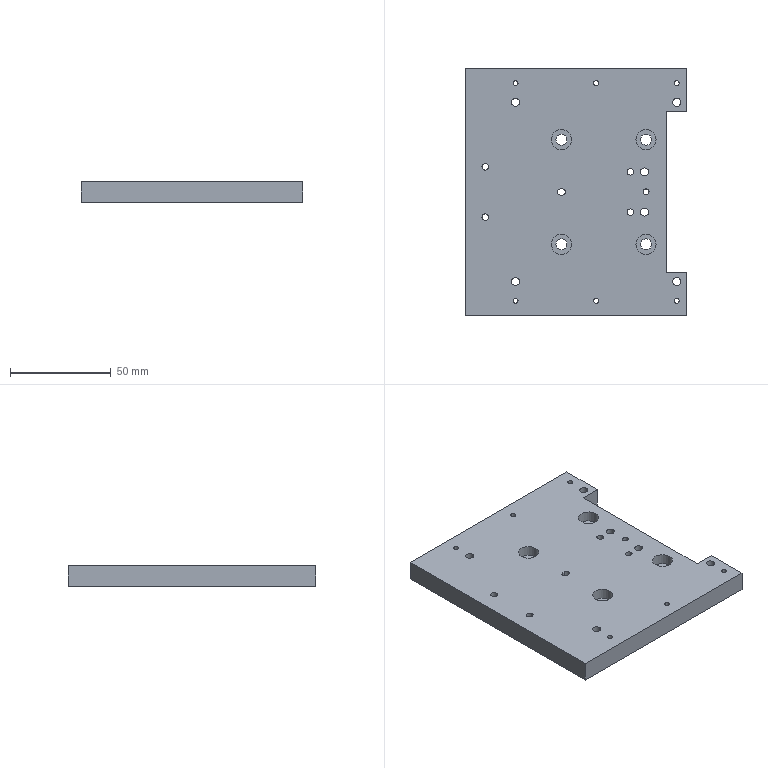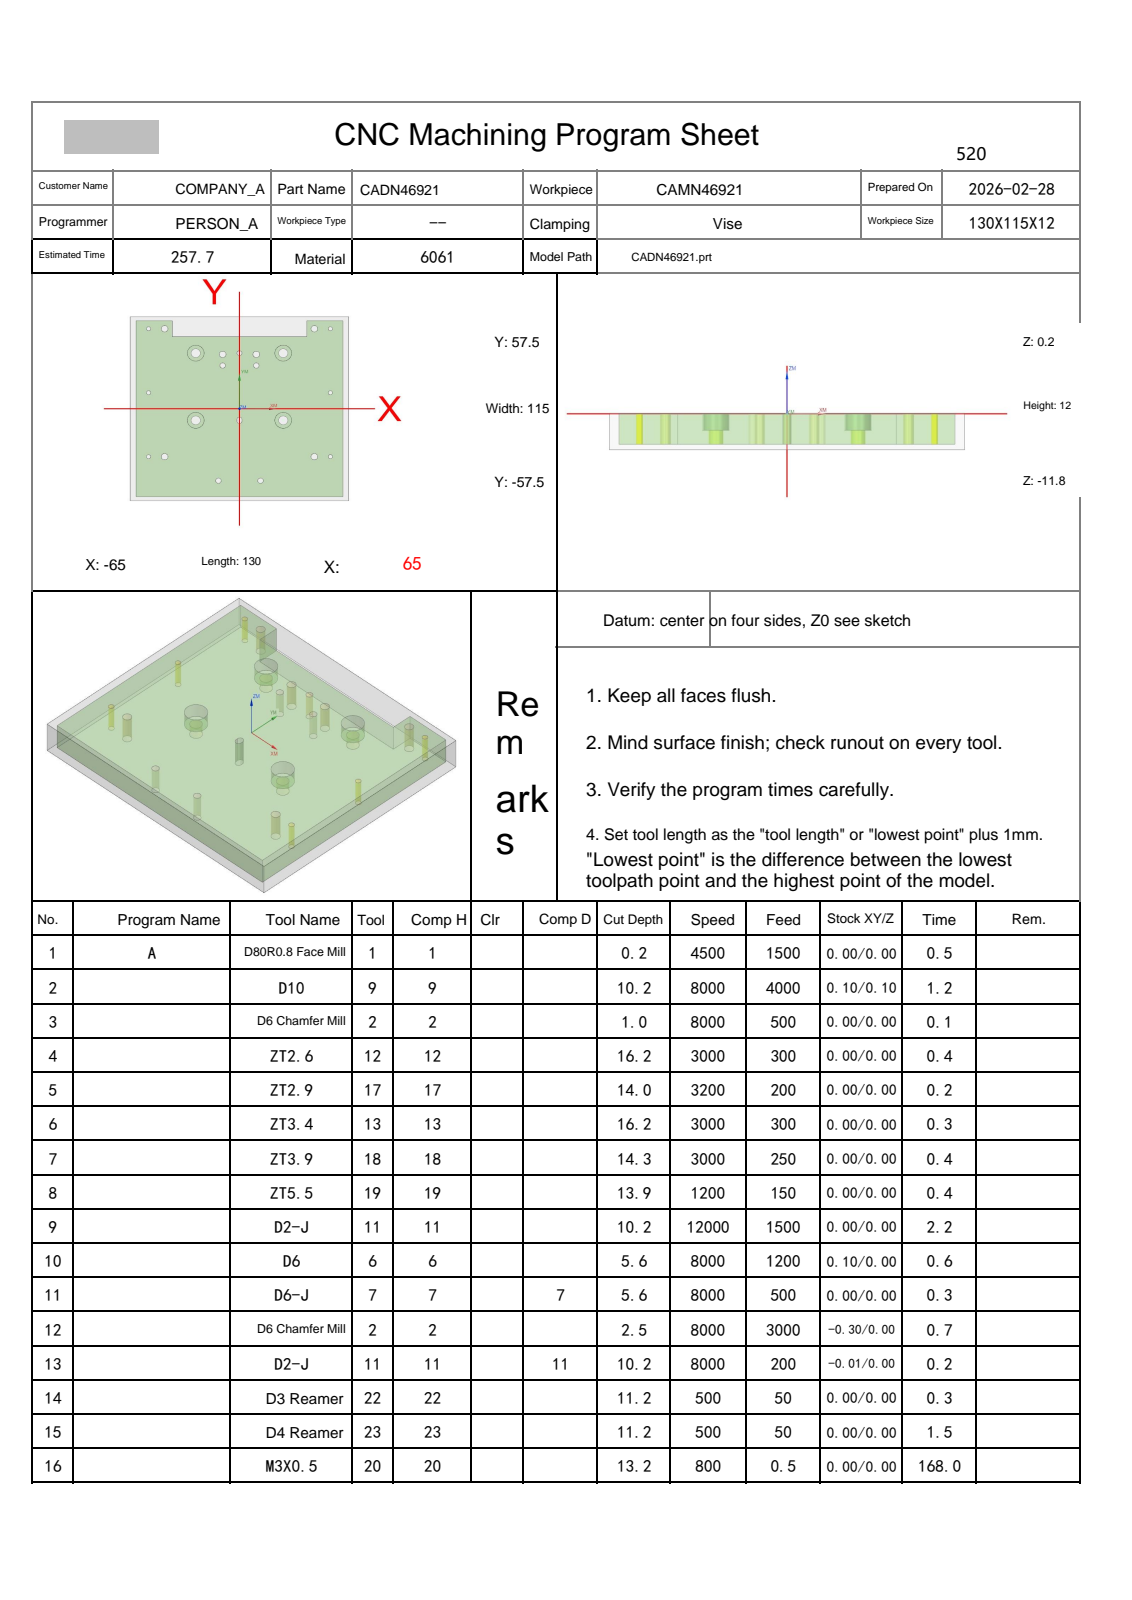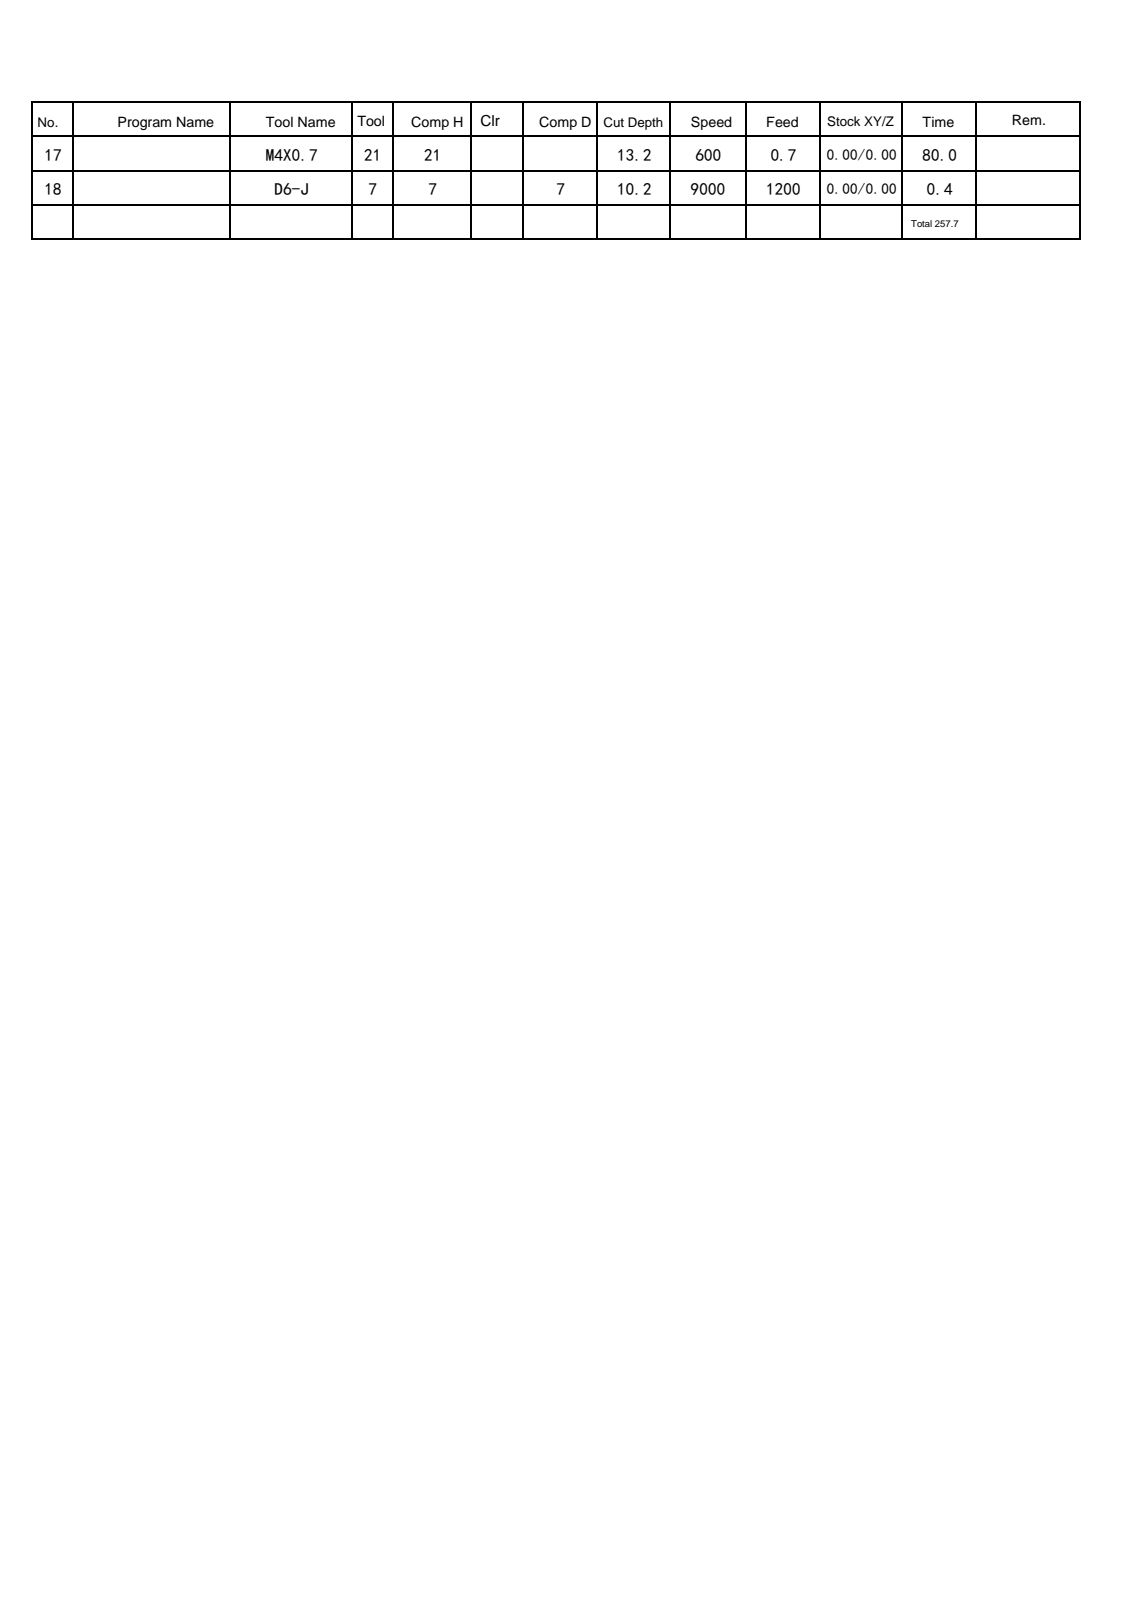NC program | NX | posted by the shop | part box 110 x 123 x 10 mm
Lines 795 to 1684 of 4511:
N9 T11 M06
(D2-J  D=2. R=0. H=11 ce=0.05 di=0.00)
G00 G90 G54 X-.45 Y-7.25 M03 S12000
G43 H11 Z50.
M08
Z.5
G01 Y-7.75 Z.49 F400.
G03 X-.307 Y-8.079 Z.482 I.45 J0.0
X0.0 Y-8.2 Z.475 I.307 J.329
X.45 Y-7.75 Z.46 I0.0 J.45
G01 Y-6.75 Z.44
G03 X0.0 Y-6.3 Z.425 I-.45 J0.0
X-.45 Y-6.75 Z.41 I0.0 J-.45
G01 Y-7.75 Z.39
G03 X-.307 Y-8.079 Z.382 I.45 J0.0
X0.0 Y-8.2 Z.375 I.307 J.329
X.45 Y-7.75 Z.36 I0.0 J.45
G01 Y-6.75 Z.34
G03 X0.0 Y-6.3 Z.325 I-.45 J0.0
X-.45 Y-6.75 Z.31 I0.0 J-.45
G01 Y-7.75 Z.29
G03 X-.307 Y-8.079 Z.282 I.45 J0.0
X0.0 Y-8.2 Z.275 I.307 J.329
X.45 Y-7.75 Z.26 I0.0 J.45
G01 Y-6.75 Z.24
G03 X0.0 Y-6.3 Z.225 I-.45 J0.0
X-.45 Y-6.75 Z.21 I0.0 J-.45
G01 Y-7.75 Z.19
G03 X-.307 Y-8.079 Z.182 I.45 J0.0
X0.0 Y-8.2 Z.175 I.307 J.329
X.45 Y-7.75 Z.16 I0.0 J.45
G01 Y-6.75 Z.14
G03 X0.0 Y-6.3 Z.125 I-.45 J0.0
X-.45 Y-6.75 Z.11 I0.0 J-.45
G01 Y-7.75 Z.09
G03 X-.307 Y-8.079 Z.082 I.45 J0.0
X0.0 Y-8.2 Z.075 I.307 J.329
X.45 Y-7.75 Z.06 I0.0 J.45
G01 Y-6.75 Z.04
G03 X0.0 Y-6.3 Z.025 I-.45 J0.0
X-.45 Y-6.75 Z.01 I0.0 J-.45
G01 Y-7.75 Z-.01
G03 X-.307 Y-8.079 Z-.018 I.45 J0.0
X0.0 Y-8.2 Z-.025 I.307 J.329
X.45 Y-7.75 Z-.04 I0.0 J.45
G01 Y-6.75 Z-.06
G03 X0.0 Y-6.3 Z-.075 I-.45 J0.0
X-.45 Y-6.75 Z-.09 I0.0 J-.45
G01 Y-7.75 Z-.11
G03 X-.307 Y-8.079 Z-.118 I.45 J0.0
X0.0 Y-8.2 Z-.125 I.307 J.329
X.45 Y-7.75 Z-.14 I0.0 J.45
G01 Y-6.75 Z-.16
G03 X0.0 Y-6.3 Z-.175 I-.45 J0.0
X-.45 Y-6.75 Z-.19 I0.0 J-.45
G01 Y-7.75 Z-.21
G03 X-.307 Y-8.079 Z-.218 I.45 J0.0
X0.0 Y-8.2 Z-.225 I.307 J.329
X.45 Y-7.75 Z-.24 I0.0 J.45
G01 Y-6.75 Z-.26
G03 X0.0 Y-6.3 Z-.275 I-.45 J0.0
X-.45 Y-6.75 Z-.29 I0.0 J-.45
G01 Y-7.75 Z-.31
G03 X-.307 Y-8.079 Z-.318 I.45 J0.0
X0.0 Y-8.2 Z-.325 I.307 J.329
X.45 Y-7.75 Z-.34 I0.0 J.45
G01 Y-6.75 Z-.36
G03 X0.0 Y-6.3 Z-.375 I-.45 J0.0
X-.45 Y-6.75 Z-.39 I0.0 J-.45
G01 Y-7.75 Z-.41
G03 X-.307 Y-8.079 Z-.418 I.45 J0.0
X0.0 Y-8.2 Z-.425 I.307 J.329
X.45 Y-7.75 Z-.44 I0.0 J.45
G01 Y-6.75 Z-.46
G03 X0.0 Y-6.3 Z-.475 I-.45 J0.0
X-.45 Y-6.75 Z-.49 I0.0 J-.45
G01 Y-7.75 Z-.51
G03 X-.307 Y-8.079 Z-.518 I.45 J0.0
X0.0 Y-8.2 Z-.525 I.307 J.329
X.45 Y-7.75 Z-.54 I0.0 J.45
G01 Y-6.75 Z-.56
G03 X0.0 Y-6.3 Z-.575 I-.45 J0.0
X-.45 Y-6.75 Z-.59 I0.0 J-.45
G01 Y-7.75 Z-.61
G03 X-.307 Y-8.079 Z-.618 I.45 J0.0
X0.0 Y-8.2 Z-.625 I.307 J.329
X.45 Y-7.75 Z-.64 I0.0 J.45
G01 Y-6.75 Z-.66
G03 X0.0 Y-6.3 Z-.675 I-.45 J0.0
X-.45 Y-6.75 Z-.69 I0.0 J-.45
G01 Y-7.75 Z-.71
G03 X-.307 Y-8.079 Z-.718 I.45 J0.0
X0.0 Y-8.2 Z-.725 I.307 J.329
X.45 Y-7.75 Z-.74 I0.0 J.45
G01 Y-6.75 Z-.76
G03 X0.0 Y-6.3 Z-.775 I-.45 J0.0
X-.45 Y-6.75 Z-.79 I0.0 J-.45
G01 Y-7.75 Z-.81
G03 X-.307 Y-8.079 Z-.818 I.45 J0.0
X0.0 Y-8.2 Z-.825 I.307 J.329
X.45 Y-7.75 Z-.84 I0.0 J.45
G01 Y-6.75 Z-.86
G03 X0.0 Y-6.3 Z-.875 I-.45 J0.0
X-.45 Y-6.75 Z-.89 I0.0 J-.45
G01 Y-7.75 Z-.91
G03 X-.307 Y-8.079 Z-.918 I.45 J0.0
X0.0 Y-8.2 Z-.925 I.307 J.329
X.45 Y-7.75 Z-.94 I0.0 J.45
G01 Y-6.75 Z-.96
G03 X0.0 Y-6.3 Z-.975 I-.45 J0.0
X-.45 Y-6.75 Z-.99 I0.0 J-.45
G01 Y-7.75 Z-1.01
G03 X-.307 Y-8.079 Z-1.018 I.45 J0.0
X0.0 Y-8.2 Z-1.025 I.307 J.329
X.45 Y-7.75 Z-1.04 I0.0 J.45
G01 Y-6.75 Z-1.06
G03 X0.0 Y-6.3 Z-1.075 I-.45 J0.0
X-.45 Y-6.75 Z-1.09 I0.0 J-.45
G01 Y-7.75 Z-1.11
G03 X-.307 Y-8.079 Z-1.118 I.45 J0.0
X0.0 Y-8.2 Z-1.125 I.307 J.329
X.45 Y-7.75 Z-1.14 I0.0 J.45
G01 Y-6.75 Z-1.16
G03 X0.0 Y-6.3 Z-1.175 I-.45 J0.0
X-.45 Y-6.75 Z-1.19 I0.0 J-.45
G01 Y-7.75 Z-1.21
G03 X-.307 Y-8.079 Z-1.218 I.45 J0.0
X0.0 Y-8.2 Z-1.225 I.307 J.329
X.45 Y-7.75 Z-1.24 I0.0 J.45
G01 Y-6.75 Z-1.26
G03 X0.0 Y-6.3 Z-1.275 I-.45 J0.0
X-.45 Y-6.75 Z-1.29 I0.0 J-.45
G01 Y-7.75 Z-1.31
G03 X-.307 Y-8.079 Z-1.318 I.45 J0.0
X0.0 Y-8.2 Z-1.325 I.307 J.329
X.45 Y-7.75 Z-1.34 I0.0 J.45
G01 Y-6.75 Z-1.36
G03 X0.0 Y-6.3 Z-1.375 I-.45 J0.0
X-.45 Y-6.75 Z-1.39 I0.0 J-.45
G01 Y-7.75 Z-1.41
G03 X-.307 Y-8.079 Z-1.418 I.45 J0.0
X0.0 Y-8.2 Z-1.425 I.307 J.329
X.45 Y-7.75 Z-1.44 I0.0 J.45
G01 Y-6.75 Z-1.46
G03 X0.0 Y-6.3 Z-1.475 I-.45 J0.0
X-.45 Y-6.75 Z-1.49 I0.0 J-.45
G01 Y-7.75 Z-1.51
G03 X-.307 Y-8.079 Z-1.518 I.45 J0.0
X0.0 Y-8.2 Z-1.525 I.307 J.329
X.45 Y-7.75 Z-1.54 I0.0 J.45
G01 Y-6.75 Z-1.56
G03 X0.0 Y-6.3 Z-1.575 I-.45 J0.0
X-.45 Y-6.75 Z-1.59 I0.0 J-.45
G01 Y-7.75 Z-1.61
G03 X-.307 Y-8.079 Z-1.618 I.45 J0.0
X0.0 Y-8.2 Z-1.625 I.307 J.329
X.45 Y-7.75 Z-1.64 I0.0 J.45
G01 Y-6.75 Z-1.66
G03 X0.0 Y-6.3 Z-1.675 I-.45 J0.0
X-.45 Y-6.75 Z-1.69 I0.0 J-.45
G01 Y-7.75 Z-1.71
G03 X-.307 Y-8.079 Z-1.718 I.45 J0.0
X0.0 Y-8.2 Z-1.725 I.307 J.329
X.45 Y-7.75 Z-1.74 I0.0 J.45
G01 Y-6.75 Z-1.76
G03 X0.0 Y-6.3 Z-1.775 I-.45 J0.0
X-.45 Y-6.75 Z-1.79 I0.0 J-.45
G01 Y-7.75 Z-1.81
G03 X-.307 Y-8.079 Z-1.818 I.45 J0.0
X0.0 Y-8.2 Z-1.825 I.307 J.329
X.45 Y-7.75 Z-1.84 I0.0 J.45
G01 Y-6.75 Z-1.86
G03 X0.0 Y-6.3 Z-1.875 I-.45 J0.0
X-.45 Y-6.75 Z-1.89 I0.0 J-.45
G01 Y-7.75 Z-1.91
G03 X-.307 Y-8.079 Z-1.918 I.45 J0.0
X0.0 Y-8.2 Z-1.925 I.307 J.329
X.45 Y-7.75 Z-1.94 I0.0 J.45
G01 Y-6.75 Z-1.96
G03 X0.0 Y-6.3 Z-1.975 I-.45 J0.0
X-.45 Y-6.75 Z-1.99 I0.0 J-.45
G01 Y-7.75 Z-2.01
G03 X-.307 Y-8.079 Z-2.018 I.45 J0.0
X0.0 Y-8.2 Z-2.025 I.307 J.329
X.45 Y-7.75 Z-2.04 I0.0 J.45
G01 Y-6.75 Z-2.06
G03 X0.0 Y-6.3 Z-2.075 I-.45 J0.0
X-.45 Y-6.75 Z-2.09 I0.0 J-.45
G01 Y-7.75 Z-2.11
G03 X-.307 Y-8.079 Z-2.118 I.45 J0.0
X0.0 Y-8.2 Z-2.125 I.307 J.329
X.45 Y-7.75 Z-2.14 I0.0 J.45
G01 Y-6.75 Z-2.16
G03 X0.0 Y-6.3 Z-2.175 I-.45 J0.0
X-.45 Y-6.75 Z-2.19 I0.0 J-.45
G01 Y-7.75 Z-2.21
G03 X-.307 Y-8.079 Z-2.218 I.45 J0.0
X0.0 Y-8.2 Z-2.225 I.307 J.329
X.45 Y-7.75 Z-2.24 I0.0 J.45
G01 Y-6.75 Z-2.26
G03 X0.0 Y-6.3 Z-2.275 I-.45 J0.0
X-.45 Y-6.75 Z-2.29 I0.0 J-.45
G01 Y-7.75 Z-2.31
G03 X-.307 Y-8.079 Z-2.318 I.45 J0.0
X0.0 Y-8.2 Z-2.325 I.307 J.329
X.45 Y-7.75 Z-2.34 I0.0 J.45
G01 Y-6.75 Z-2.36
G03 X0.0 Y-6.3 Z-2.375 I-.45 J0.0
X-.45 Y-6.75 Z-2.39 I0.0 J-.45
G01 Y-7.75 Z-2.41
G03 X-.307 Y-8.079 Z-2.418 I.45 J0.0
X0.0 Y-8.2 Z-2.425 I.307 J.329
X.45 Y-7.75 Z-2.44 I0.0 J.45
G01 Y-6.75 Z-2.46
G03 X0.0 Y-6.3 Z-2.475 I-.45 J0.0
X-.45 Y-6.75 Z-2.49 I0.0 J-.45
G01 Y-7.75 Z-2.51
G03 X-.307 Y-8.079 Z-2.518 I.45 J0.0
X0.0 Y-8.2 Z-2.525 I.307 J.329
X.45 Y-7.75 Z-2.54 I0.0 J.45
G01 Y-6.75 Z-2.56
G03 X0.0 Y-6.3 Z-2.575 I-.45 J0.0
X-.45 Y-6.75 Z-2.59 I0.0 J-.45
G01 Y-7.75 Z-2.61
G03 X-.307 Y-8.079 Z-2.618 I.45 J0.0
X0.0 Y-8.2 Z-2.625 I.307 J.329
X.45 Y-7.75 Z-2.64 I0.0 J.45
G01 Y-6.75 Z-2.66
G03 X0.0 Y-6.3 Z-2.675 I-.45 J0.0
X-.45 Y-6.75 Z-2.69 I0.0 J-.45
G01 Y-7.75 Z-2.71
G03 X-.307 Y-8.079 Z-2.718 I.45 J0.0
X0.0 Y-8.2 Z-2.725 I.307 J.329
X.45 Y-7.75 Z-2.74 I0.0 J.45
G01 Y-6.75 Z-2.76
G03 X0.0 Y-6.3 Z-2.775 I-.45 J0.0
X-.45 Y-6.75 Z-2.79 I0.0 J-.45
G01 Y-7.75 Z-2.81
G03 X-.307 Y-8.079 Z-2.818 I.45 J0.0
X0.0 Y-8.2 Z-2.825 I.307 J.329
X.45 Y-7.75 Z-2.84 I0.0 J.45
G01 Y-6.75 Z-2.86
G03 X0.0 Y-6.3 Z-2.875 I-.45 J0.0
X-.45 Y-6.75 Z-2.89 I0.0 J-.45
G01 Y-7.75 Z-2.91
G03 X-.307 Y-8.079 Z-2.918 I.45 J0.0
X0.0 Y-8.2 Z-2.925 I.307 J.329
X.45 Y-7.75 Z-2.94 I0.0 J.45
G01 Y-6.75 Z-2.96
G03 X0.0 Y-6.3 Z-2.975 I-.45 J0.0
X-.45 Y-6.75 Z-2.99 I0.0 J-.45
G01 Y-7.75 Z-3.01
G03 X-.307 Y-8.079 Z-3.018 I.45 J0.0
X0.0 Y-8.2 Z-3.025 I.307 J.329
X.45 Y-7.75 Z-3.04 I0.0 J.45
G01 Y-6.75 Z-3.06
G03 X0.0 Y-6.3 Z-3.075 I-.45 J0.0
X-.45 Y-6.75 Z-3.09 I0.0 J-.45
G01 Y-7.75 Z-3.11
G03 X-.307 Y-8.079 Z-3.118 I.45 J0.0
X0.0 Y-8.2 Z-3.125 I.307 J.329
X.45 Y-7.75 Z-3.14 I0.0 J.45
G01 Y-6.75 Z-3.16
G03 X0.0 Y-6.3 Z-3.175 I-.45 J0.0
X-.45 Y-6.75 Z-3.19 I0.0 J-.45
G01 Y-7.75 Z-3.21
G03 X-.307 Y-8.079 Z-3.218 I.45 J0.0
X0.0 Y-8.2 Z-3.225 I.307 J.329
X.45 Y-7.75 Z-3.24 I0.0 J.45
G01 Y-6.75 Z-3.26
G03 X0.0 Y-6.3 Z-3.275 I-.45 J0.0
X-.45 Y-6.75 Z-3.29 I0.0 J-.45
G01 Y-7.75 Z-3.31
G03 X-.307 Y-8.079 Z-3.318 I.45 J0.0
X0.0 Y-8.2 Z-3.325 I.307 J.329
X.45 Y-7.75 Z-3.34 I0.0 J.45
G01 Y-6.75 Z-3.36
G03 X0.0 Y-6.3 Z-3.375 I-.45 J0.0
X-.45 Y-6.75 Z-3.39 I0.0 J-.45
G01 Y-7.75 Z-3.41
G03 X-.307 Y-8.079 Z-3.418 I.45 J0.0
X0.0 Y-8.2 Z-3.425 I.307 J.329
X.45 Y-7.75 Z-3.44 I0.0 J.45
G01 Y-6.75 Z-3.46
G03 X0.0 Y-6.3 Z-3.475 I-.45 J0.0
X-.45 Y-6.75 Z-3.49 I0.0 J-.45
G01 Y-7.75 Z-3.51
G03 X-.307 Y-8.079 Z-3.518 I.45 J0.0
X0.0 Y-8.2 Z-3.525 I.307 J.329
X.45 Y-7.75 Z-3.54 I0.0 J.45
G01 Y-6.75 Z-3.56
G03 X0.0 Y-6.3 Z-3.575 I-.45 J0.0
X-.45 Y-6.75 Z-3.59 I0.0 J-.45
G01 Y-7.75 Z-3.61
G03 X-.307 Y-8.079 Z-3.618 I.45 J0.0
X0.0 Y-8.2 Z-3.625 I.307 J.329
X.45 Y-7.75 Z-3.64 I0.0 J.45
G01 Y-6.75 Z-3.66
G03 X0.0 Y-6.3 Z-3.675 I-.45 J0.0
X-.45 Y-6.75 Z-3.69 I0.0 J-.45
G01 Y-7.75 Z-3.71
G03 X-.307 Y-8.079 Z-3.718 I.45 J0.0
X0.0 Y-8.2 Z-3.725 I.307 J.329
X.45 Y-7.75 Z-3.74 I0.0 J.45
G01 Y-6.75 Z-3.76
G03 X0.0 Y-6.3 Z-3.775 I-.45 J0.0
X-.45 Y-6.75 Z-3.79 I0.0 J-.45
G01 Y-7.75 Z-3.81
G03 X-.307 Y-8.079 Z-3.818 I.45 J0.0
X0.0 Y-8.2 Z-3.825 I.307 J.329
X.45 Y-7.75 Z-3.84 I0.0 J.45
G01 Y-6.75 Z-3.86
G03 X0.0 Y-6.3 Z-3.875 I-.45 J0.0
X-.45 Y-6.75 Z-3.89 I0.0 J-.45
G01 Y-7.75 Z-3.91
G03 X-.307 Y-8.079 Z-3.918 I.45 J0.0
X0.0 Y-8.2 Z-3.925 I.307 J.329
X.45 Y-7.75 Z-3.94 I0.0 J.45
G01 Y-6.75 Z-3.96
G03 X0.0 Y-6.3 Z-3.975 I-.45 J0.0
X-.45 Y-6.75 Z-3.99 I0.0 J-.45
G01 Y-7.75 Z-4.01
G03 X-.307 Y-8.079 Z-4.018 I.45 J0.0
X0.0 Y-8.2 Z-4.025 I.307 J.329
X.45 Y-7.75 Z-4.04 I0.0 J.45
G01 Y-6.75 Z-4.06
G03 X0.0 Y-6.3 Z-4.075 I-.45 J0.0
X-.45 Y-6.75 Z-4.09 I0.0 J-.45
G01 Y-7.75 Z-4.11
G03 X-.307 Y-8.079 Z-4.118 I.45 J0.0
X0.0 Y-8.2 Z-4.125 I.307 J.329
X.45 Y-7.75 Z-4.14 I0.0 J.45
G01 Y-6.75 Z-4.16
G03 X0.0 Y-6.3 Z-4.175 I-.45 J0.0
X-.45 Y-6.75 Z-4.19 I0.0 J-.45
G01 Y-7.75 Z-4.21
G03 X-.307 Y-8.079 Z-4.218 I.45 J0.0
X0.0 Y-8.2 Z-4.225 I.307 J.329
X.45 Y-7.75 Z-4.24 I0.0 J.45
G01 Y-6.75 Z-4.26
G03 X0.0 Y-6.3 Z-4.275 I-.45 J0.0
X-.45 Y-6.75 Z-4.29 I0.0 J-.45
G01 Y-7.75 Z-4.31
G03 X-.307 Y-8.079 Z-4.318 I.45 J0.0
X0.0 Y-8.2 Z-4.325 I.307 J.329
X.45 Y-7.75 Z-4.34 I0.0 J.45
G01 Y-6.75 Z-4.36
G03 X0.0 Y-6.3 Z-4.375 I-.45 J0.0
X-.45 Y-6.75 Z-4.39 I0.0 J-.45
G01 Y-7.75 Z-4.41
G03 X-.307 Y-8.079 Z-4.418 I.45 J0.0
X0.0 Y-8.2 Z-4.425 I.307 J.329
X.45 Y-7.75 Z-4.44 I0.0 J.45
G01 Y-6.75 Z-4.46
G03 X0.0 Y-6.3 Z-4.475 I-.45 J0.0
X-.45 Y-6.75 Z-4.49 I0.0 J-.45
G01 Y-7.75 Z-4.51
G03 X-.307 Y-8.079 Z-4.518 I.45 J0.0
X0.0 Y-8.2 Z-4.525 I.307 J.329
X.45 Y-7.75 Z-4.54 I0.0 J.45
G01 Y-6.75 Z-4.56
G03 X0.0 Y-6.3 Z-4.575 I-.45 J0.0
X-.45 Y-6.75 Z-4.59 I0.0 J-.45
G01 Y-7.75 Z-4.61
G03 X-.307 Y-8.079 Z-4.618 I.45 J0.0
X0.0 Y-8.2 Z-4.625 I.307 J.329
X.45 Y-7.75 Z-4.64 I0.0 J.45
G01 Y-6.75 Z-4.66
G03 X0.0 Y-6.3 Z-4.675 I-.45 J0.0
X-.45 Y-6.75 Z-4.69 I0.0 J-.45
G01 Y-7.75 Z-4.71
G03 X-.307 Y-8.079 Z-4.718 I.45 J0.0
X0.0 Y-8.2 Z-4.725 I.307 J.329
X.45 Y-7.75 Z-4.74 I0.0 J.45
G01 Y-6.75 Z-4.76
G03 X0.0 Y-6.3 Z-4.775 I-.45 J0.0
X-.45 Y-6.75 Z-4.79 I0.0 J-.45
G01 Y-7.75 Z-4.81
G03 X-.307 Y-8.079 Z-4.818 I.45 J0.0
X0.0 Y-8.2 Z-4.825 I.307 J.329
X.45 Y-7.75 Z-4.84 I0.0 J.45
G01 Y-6.75 Z-4.86
G03 X0.0 Y-6.3 Z-4.875 I-.45 J0.0
X-.45 Y-6.75 Z-4.89 I0.0 J-.45
G01 Y-7.75 Z-4.91
G03 X-.307 Y-8.079 Z-4.918 I.45 J0.0
X0.0 Y-8.2 Z-4.925 I.307 J.329
X.45 Y-7.75 Z-4.94 I0.0 J.45
G01 Y-6.75 Z-4.96
G03 X0.0 Y-6.3 Z-4.975 I-.45 J0.0
X-.45 Y-6.75 Z-4.99 I0.0 J-.45
G01 Y-7.75 Z-5.01
G03 X-.307 Y-8.079 Z-5.018 I.45 J0.0
X0.0 Y-8.2 Z-5.025 I.307 J.329
X.45 Y-7.75 Z-5.04 I0.0 J.45
G01 Y-6.75 Z-5.06
G03 X0.0 Y-6.3 Z-5.075 I-.45 J0.0
X-.45 Y-6.75 Z-5.09 I0.0 J-.45
G01 Y-7.75 Z-5.11
G03 X-.307 Y-8.079 Z-5.118 I.45 J0.0
X0.0 Y-8.2 Z-5.125 I.307 J.329
X.45 Y-7.75 Z-5.14 I0.0 J.45
G01 Y-6.75 Z-5.16
G03 X0.0 Y-6.3 Z-5.175 I-.45 J0.0
X-.45 Y-6.75 Z-5.19 I0.0 J-.45
G01 Y-7.75 Z-5.21
G03 X-.307 Y-8.079 Z-5.218 I.45 J0.0
X0.0 Y-8.2 Z-5.225 I.307 J.329
X.45 Y-7.75 Z-5.24 I0.0 J.45
G01 Y-6.75 Z-5.26
G03 X0.0 Y-6.3 Z-5.275 I-.45 J0.0
X-.45 Y-6.75 Z-5.29 I0.0 J-.45
G01 Y-7.75 Z-5.31
G03 X-.307 Y-8.079 Z-5.318 I.45 J0.0
X0.0 Y-8.2 Z-5.325 I.307 J.329
X.45 Y-7.75 Z-5.34 I0.0 J.45
G01 Y-6.75 Z-5.36
G03 X0.0 Y-6.3 Z-5.375 I-.45 J0.0
X-.45 Y-6.75 Z-5.39 I0.0 J-.45
G01 Y-7.75 Z-5.41
G03 X-.307 Y-8.079 Z-5.418 I.45 J0.0
X0.0 Y-8.2 Z-5.425 I.307 J.329
X.45 Y-7.75 Z-5.44 I0.0 J.45
G01 Y-6.75 Z-5.46
G03 X0.0 Y-6.3 Z-5.475 I-.45 J0.0
X-.45 Y-6.75 Z-5.49 I0.0 J-.45
G01 Y-7.75 Z-5.51
G03 X-.307 Y-8.079 Z-5.518 I.45 J0.0
X0.0 Y-8.2 Z-5.525 I.307 J.329
X.45 Y-7.75 Z-5.54 I0.0 J.45
G01 Y-6.75 Z-5.56
G03 X0.0 Y-6.3 Z-5.575 I-.45 J0.0
X-.45 Y-6.75 Z-5.59 I0.0 J-.45
G01 Y-7.75 Z-5.61
G03 X-.307 Y-8.079 Z-5.618 I.45 J0.0
X0.0 Y-8.2 Z-5.625 I.307 J.329
X.45 Y-7.75 Z-5.64 I0.0 J.45
G01 Y-6.75 Z-5.66
G03 X0.0 Y-6.3 Z-5.675 I-.45 J0.0
X-.45 Y-6.75 Z-5.69 I0.0 J-.45
G01 Y-7.75 Z-5.71
G03 X-.307 Y-8.079 Z-5.718 I.45 J0.0
X0.0 Y-8.2 Z-5.725 I.307 J.329
X.45 Y-7.75 Z-5.74 I0.0 J.45
G01 Y-6.75 Z-5.76
G03 X0.0 Y-6.3 Z-5.775 I-.45 J0.0
X-.45 Y-6.75 Z-5.79 I0.0 J-.45
G01 Y-7.75 Z-5.81
G03 X-.307 Y-8.079 Z-5.818 I.45 J0.0
X0.0 Y-8.2 Z-5.825 I.307 J.329
X.45 Y-7.75 Z-5.84 I0.0 J.45
G01 Y-6.75 Z-5.86
G03 X0.0 Y-6.3 Z-5.875 I-.45 J0.0
X-.45 Y-6.75 Z-5.89 I0.0 J-.45
G01 Y-7.75 Z-5.91
G03 X-.307 Y-8.079 Z-5.918 I.45 J0.0
X0.0 Y-8.2 Z-5.925 I.307 J.329
X.45 Y-7.75 Z-5.94 I0.0 J.45
G01 Y-6.75 Z-5.96
G03 X0.0 Y-6.3 Z-5.975 I-.45 J0.0
X-.45 Y-6.75 Z-5.99 I0.0 J-.45
G01 Y-7.75 Z-6.01
G03 X-.307 Y-8.079 Z-6.018 I.45 J0.0
X0.0 Y-8.2 Z-6.025 I.307 J.329
X.45 Y-7.75 Z-6.04 I0.0 J.45
G01 Y-6.75 Z-6.06
G03 X0.0 Y-6.3 Z-6.075 I-.45 J0.0
X-.45 Y-6.75 Z-6.09 I0.0 J-.45
G01 Y-7.75 Z-6.11
G03 X-.307 Y-8.079 Z-6.118 I.45 J0.0
X0.0 Y-8.2 Z-6.125 I.307 J.329
X.45 Y-7.75 Z-6.14 I0.0 J.45
G01 Y-6.75 Z-6.16
G03 X0.0 Y-6.3 Z-6.175 I-.45 J0.0
X-.45 Y-6.75 Z-6.19 I0.0 J-.45
G01 Y-7.75 Z-6.21
G03 X-.307 Y-8.079 Z-6.218 I.45 J0.0
X0.0 Y-8.2 Z-6.225 I.307 J.329
X.45 Y-7.75 Z-6.24 I0.0 J.45
G01 Y-6.75 Z-6.26
G03 X0.0 Y-6.3 Z-6.275 I-.45 J0.0
X-.45 Y-6.75 Z-6.29 I0.0 J-.45
G01 Y-7.75 Z-6.31
G03 X-.307 Y-8.079 Z-6.318 I.45 J0.0
X0.0 Y-8.2 Z-6.325 I.307 J.329
X.45 Y-7.75 Z-6.34 I0.0 J.45
G01 Y-6.75 Z-6.36
G03 X0.0 Y-6.3 Z-6.375 I-.45 J0.0
X-.45 Y-6.75 Z-6.39 I0.0 J-.45
G01 Y-7.75 Z-6.41
G03 X-.307 Y-8.079 Z-6.418 I.45 J0.0
X0.0 Y-8.2 Z-6.425 I.307 J.329
X.45 Y-7.75 Z-6.44 I0.0 J.45
G01 Y-6.75 Z-6.46
G03 X0.0 Y-6.3 Z-6.475 I-.45 J0.0
X-.45 Y-6.75 Z-6.49 I0.0 J-.45
G01 Y-7.75 Z-6.51
G03 X-.307 Y-8.079 Z-6.518 I.45 J0.0
X0.0 Y-8.2 Z-6.525 I.307 J.329
X.45 Y-7.75 Z-6.54 I0.0 J.45
G01 Y-6.75 Z-6.56
G03 X0.0 Y-6.3 Z-6.575 I-.45 J0.0
X-.45 Y-6.75 Z-6.59 I0.0 J-.45
G01 Y-7.75 Z-6.61
G03 X-.307 Y-8.079 Z-6.618 I.45 J0.0
X0.0 Y-8.2 Z-6.625 I.307 J.329
X.45 Y-7.75 Z-6.64 I0.0 J.45
G01 Y-6.75 Z-6.66
G03 X0.0 Y-6.3 Z-6.675 I-.45 J0.0
X-.45 Y-6.75 Z-6.69 I0.0 J-.45
G01 Y-7.75 Z-6.71
G03 X-.307 Y-8.079 Z-6.718 I.45 J0.0
X0.0 Y-8.2 Z-6.725 I.307 J.329
X.45 Y-7.75 Z-6.74 I0.0 J.45
G01 Y-6.75 Z-6.76
G03 X0.0 Y-6.3 Z-6.775 I-.45 J0.0
X-.45 Y-6.75 Z-6.79 I0.0 J-.45
G01 Y-7.75 Z-6.81
G03 X-.307 Y-8.079 Z-6.818 I.45 J0.0
X0.0 Y-8.2 Z-6.825 I.307 J.329
X.45 Y-7.75 Z-6.84 I0.0 J.45
G01 Y-6.75 Z-6.86
G03 X0.0 Y-6.3 Z-6.875 I-.45 J0.0
X-.45 Y-6.75 Z-6.89 I0.0 J-.45
G01 Y-7.75 Z-6.91
G03 X-.307 Y-8.079 Z-6.918 I.45 J0.0
X0.0 Y-8.2 Z-6.925 I.307 J.329
X.45 Y-7.75 Z-6.94 I0.0 J.45
G01 Y-6.75 Z-6.96
G03 X0.0 Y-6.3 Z-6.975 I-.45 J0.0
X-.45 Y-6.75 Z-6.99 I0.0 J-.45
G01 Y-7.75 Z-7.01
G03 X-.307 Y-8.079 Z-7.018 I.45 J0.0
X0.0 Y-8.2 Z-7.025 I.307 J.329
X.45 Y-7.75 Z-7.04 I0.0 J.45
G01 Y-6.75 Z-7.06
G03 X0.0 Y-6.3 Z-7.075 I-.45 J0.0
X-.45 Y-6.75 Z-7.09 I0.0 J-.45
G01 Y-7.75 Z-7.11
G03 X-.307 Y-8.079 Z-7.118 I.45 J0.0
X0.0 Y-8.2 Z-7.125 I.307 J.329
X.45 Y-7.75 Z-7.14 I0.0 J.45
G01 Y-6.75 Z-7.16
G03 X0.0 Y-6.3 Z-7.175 I-.45 J0.0
X-.45 Y-6.75 Z-7.19 I0.0 J-.45
G01 Y-7.75 Z-7.21
G03 X-.307 Y-8.079 Z-7.218 I.45 J0.0
X0.0 Y-8.2 Z-7.225 I.307 J.329
X.45 Y-7.75 Z-7.24 I0.0 J.45
G01 Y-6.75 Z-7.26
G03 X0.0 Y-6.3 Z-7.275 I-.45 J0.0
X-.45 Y-6.75 Z-7.29 I0.0 J-.45
G01 Y-7.75 Z-7.31
G03 X-.307 Y-8.079 Z-7.318 I.45 J0.0
X0.0 Y-8.2 Z-7.325 I.307 J.329
X.45 Y-7.75 Z-7.34 I0.0 J.45
G01 Y-6.75 Z-7.36
G03 X0.0 Y-6.3 Z-7.375 I-.45 J0.0
X-.45 Y-6.75 Z-7.39 I0.0 J-.45
G01 Y-7.75 Z-7.41
G03 X-.307 Y-8.079 Z-7.418 I.45 J0.0
X0.0 Y-8.2 Z-7.425 I.307 J.329
X.45 Y-7.75 Z-7.44 I0.0 J.45
G01 Y-6.75 Z-7.46
G03 X0.0 Y-6.3 Z-7.475 I-.45 J0.0
X-.45 Y-6.75 Z-7.49 I0.0 J-.45
G01 Y-7.75 Z-7.51
G03 X-.307 Y-8.079 Z-7.518 I.45 J0.0
X0.0 Y-8.2 Z-7.525 I.307 J.329
X.45 Y-7.75 Z-7.54 I0.0 J.45
G01 Y-6.75 Z-7.56
G03 X0.0 Y-6.3 Z-7.575 I-.45 J0.0
X-.45 Y-6.75 Z-7.59 I0.0 J-.45
G01 Y-7.75 Z-7.61
G03 X-.307 Y-8.079 Z-7.618 I.45 J0.0
X0.0 Y-8.2 Z-7.625 I.307 J.329
X.45 Y-7.75 Z-7.64 I0.0 J.45
G01 Y-6.75 Z-7.66
G03 X0.0 Y-6.3 Z-7.675 I-.45 J0.0
X-.45 Y-6.75 Z-7.69 I0.0 J-.45
G01 Y-7.75 Z-7.71
G03 X-.307 Y-8.079 Z-7.718 I.45 J0.0
X0.0 Y-8.2 Z-7.725 I.307 J.329
X.45 Y-7.75 Z-7.74 I0.0 J.45
G01 Y-6.75 Z-7.76
G03 X0.0 Y-6.3 Z-7.775 I-.45 J0.0
X-.45 Y-6.75 Z-7.79 I0.0 J-.45
G01 Y-7.75 Z-7.81
G03 X-.307 Y-8.079 Z-7.818 I.45 J0.0
X0.0 Y-8.2 Z-7.825 I.307 J.329
X.45 Y-7.75 Z-7.84 I0.0 J.45
G01 Y-6.75 Z-7.86
G03 X0.0 Y-6.3 Z-7.875 I-.45 J0.0
X-.45 Y-6.75 Z-7.89 I0.0 J-.45
G01 Y-7.75 Z-7.91
G03 X-.307 Y-8.079 Z-7.918 I.45 J0.0
X0.0 Y-8.2 Z-7.925 I.307 J.329
X.45 Y-7.75 Z-7.94 I0.0 J.45
G01 Y-6.75 Z-7.96
G03 X0.0 Y-6.3 Z-7.975 I-.45 J0.0
X-.45 Y-6.75 Z-7.99 I0.0 J-.45
G01 Y-7.75 Z-8.01
G03 X-.307 Y-8.079 Z-8.018 I.45 J0.0
X0.0 Y-8.2 Z-8.025 I.307 J.329
X.45 Y-7.75 Z-8.04 I0.0 J.45
G01 Y-6.75 Z-8.06
G03 X0.0 Y-6.3 Z-8.075 I-.45 J0.0
X-.45 Y-6.75 Z-8.09 I0.0 J-.45
G01 Y-7.75 Z-8.11
G03 X-.307 Y-8.079 Z-8.118 I.45 J0.0
X0.0 Y-8.2 Z-8.125 I.307 J.329
X.45 Y-7.75 Z-8.14 I0.0 J.45
G01 Y-6.75 Z-8.16
G03 X0.0 Y-6.3 Z-8.175 I-.45 J0.0
X-.45 Y-6.75 Z-8.19 I0.0 J-.45
G01 Y-7.75 Z-8.21
G03 X-.307 Y-8.079 Z-8.218 I.45 J0.0
X0.0 Y-8.2 Z-8.225 I.307 J.329
X.45 Y-7.75 Z-8.24 I0.0 J.45
G01 Y-6.75 Z-8.26
G03 X0.0 Y-6.3 Z-8.275 I-.45 J0.0
X-.45 Y-6.75 Z-8.29 I0.0 J-.45
G01 Y-7.75 Z-8.31
G03 X-.307 Y-8.079 Z-8.318 I.45 J0.0
X0.0 Y-8.2 Z-8.325 I.307 J.329
X.45 Y-7.75 Z-8.34 I0.0 J.45
G01 Y-6.75 Z-8.36
G03 X0.0 Y-6.3 Z-8.375 I-.45 J0.0
X-.45 Y-6.75 Z-8.39 I0.0 J-.45
G01 Y-7.75 Z-8.41
G03 X-.307 Y-8.079 Z-8.418 I.45 J0.0
X0.0 Y-8.2 Z-8.425 I.307 J.329
X.45 Y-7.75 Z-8.44 I0.0 J.45
G01 Y-6.75 Z-8.46
G03 X0.0 Y-6.3 Z-8.475 I-.45 J0.0
X-.45 Y-6.75 Z-8.49 I0.0 J-.45
G01 Y-7.75 Z-8.51
G03 X-.307 Y-8.079 Z-8.518 I.45 J0.0
X0.0 Y-8.2 Z-8.525 I.307 J.329
X.45 Y-7.75 Z-8.54 I0.0 J.45
G01 Y-6.75 Z-8.56
G03 X0.0 Y-6.3 Z-8.575 I-.45 J0.0
X-.45 Y-6.75 Z-8.59 I0.0 J-.45
G01 Y-7.75 Z-8.61
G03 X-.307 Y-8.079 Z-8.618 I.45 J0.0
X0.0 Y-8.2 Z-8.625 I.307 J.329
X.45 Y-7.75 Z-8.64 I0.0 J.45
G01 Y-6.75 Z-8.66
G03 X0.0 Y-6.3 Z-8.675 I-.45 J0.0
X-.45 Y-6.75 Z-8.69 I0.0 J-.45
G01 Y-7.75 Z-8.71
G03 X-.307 Y-8.079 Z-8.718 I.45 J0.0
X0.0 Y-8.2 Z-8.725 I.307 J.329
X.45 Y-7.75 Z-8.74 I0.0 J.45
G01 Y-6.75 Z-8.76
G03 X0.0 Y-6.3 Z-8.775 I-.45 J0.0
X-.45 Y-6.75 Z-8.79 I0.0 J-.45
G01 Y-7.75 Z-8.81
G03 X-.307 Y-8.079 Z-8.818 I.45 J0.0
X0.0 Y-8.2 Z-8.825 I.307 J.329
X.45 Y-7.75 Z-8.84 I0.0 J.45
G01 Y-6.75 Z-8.86
G03 X0.0 Y-6.3 Z-8.875 I-.45 J0.0
X-.45 Y-6.75 Z-8.89 I0.0 J-.45
G01 Y-7.75 Z-8.91
G03 X-.307 Y-8.079 Z-8.918 I.45 J0.0
X0.0 Y-8.2 Z-8.925 I.307 J.329
X.45 Y-7.75 Z-8.94 I0.0 J.45
G01 Y-6.75 Z-8.96
G03 X0.0 Y-6.3 Z-8.975 I-.45 J0.0
X-.45 Y-6.75 Z-8.99 I0.0 J-.45
G01 Y-7.75 Z-9.01
G03 X-.307 Y-8.079 Z-9.018 I.45 J0.0
X0.0 Y-8.2 Z-9.025 I.307 J.329
X.45 Y-7.75 Z-9.04 I0.0 J.45
G01 Y-6.75 Z-9.06
G03 X0.0 Y-6.3 Z-9.075 I-.45 J0.0
X-.45 Y-6.75 Z-9.09 I0.0 J-.45
G01 Y-7.75 Z-9.11
G03 X-.307 Y-8.079 Z-9.118 I.45 J0.0
X0.0 Y-8.2 Z-9.125 I.307 J.329
X.45 Y-7.75 Z-9.14 I0.0 J.45
G01 Y-6.75 Z-9.16
G03 X0.0 Y-6.3 Z-9.175 I-.45 J0.0
X-.45 Y-6.75 Z-9.19 I0.0 J-.45
G01 Y-7.75 Z-9.21
G03 X-.307 Y-8.079 Z-9.218 I.45 J0.0
X0.0 Y-8.2 Z-9.225 I.307 J.329
X.45 Y-7.75 Z-9.24 I0.0 J.45
G01 Y-6.75 Z-9.26
G03 X0.0 Y-6.3 Z-9.275 I-.45 J0.0
X-.45 Y-6.75 Z-9.29 I0.0 J-.45
G01 Y-7.75 Z-9.31
G03 X-.307 Y-8.079 Z-9.318 I.45 J0.0
X0.0 Y-8.2 Z-9.325 I.307 J.329
X.45 Y-7.75 Z-9.34 I0.0 J.45
G01 Y-6.75 Z-9.36
G03 X0.0 Y-6.3 Z-9.375 I-.45 J0.0
X-.45 Y-6.75 Z-9.39 I0.0 J-.45
G01 Y-7.75 Z-9.41
G03 X-.307 Y-8.079 Z-9.418 I.45 J0.0
X0.0 Y-8.2 Z-9.425 I.307 J.329
X.45 Y-7.75 Z-9.44 I0.0 J.45
G01 Y-6.75 Z-9.46
G03 X0.0 Y-6.3 Z-9.475 I-.45 J0.0
X-.45 Y-6.75 Z-9.49 I0.0 J-.45
G01 Y-7.75 Z-9.51
G03 X-.307 Y-8.079 Z-9.518 I.45 J0.0
X0.0 Y-8.2 Z-9.525 I.307 J.329
X.45 Y-7.75 Z-9.54 I0.0 J.45
G01 Y-6.75 Z-9.56
G03 X0.0 Y-6.3 Z-9.575 I-.45 J0.0
X-.45 Y-6.75 Z-9.59 I0.0 J-.45
G01 Y-7.75 Z-9.61
G03 X-.307 Y-8.079 Z-9.618 I.45 J0.0
X0.0 Y-8.2 Z-9.625 I.307 J.329
X.45 Y-7.75 Z-9.64 I0.0 J.45
G01 Y-6.75 Z-9.66
G03 X0.0 Y-6.3 Z-9.675 I-.45 J0.0
X-.45 Y-6.75 Z-9.69 I0.0 J-.45
G01 Y-7.75 Z-9.71
G03 X-.307 Y-8.079 Z-9.718 I.45 J0.0
X0.0 Y-8.2 Z-9.725 I.307 J.329
X.45 Y-7.75 Z-9.74 I0.0 J.45
G01 Y-6.75 Z-9.76
G03 X0.0 Y-6.3 Z-9.775 I-.45 J0.0
X-.45 Y-6.75 Z-9.79 I0.0 J-.45
G01 Y-7.75 Z-9.81
G03 X-.307 Y-8.079 Z-9.818 I.45 J0.0
X0.0 Y-8.2 Z-9.825 I.307 J.329
X.45 Y-7.75 Z-9.84 I0.0 J.45
G01 Y-6.75 Z-9.86
G03 X0.0 Y-6.3 Z-9.875 I-.45 J0.0
X-.45 Y-6.75 Z-9.89 I0.0 J-.45
G01 Y-7.75 Z-9.91
G03 X-.307 Y-8.079 Z-9.918 I.45 J0.0
X0.0 Y-8.2 Z-9.925 I.307 J.329
X.45 Y-7.75 Z-9.94 I0.0 J.45
G01 Y-6.75 Z-9.96
G03 X0.0 Y-6.3 Z-9.975 I-.45 J0.0
X-.45 Y-6.75 Z-9.99 I0.0 J-.45
G01 Y-7.25 Z-10.
Y-7.75
G03 X0.0 Y-8.2 I.45 J0.0
X.45 Y-7.75 I0.0 J.45
G01 Y-6.75
G03 X0.0 Y-6.3 I-.45 J0.0
X-.45 Y-6.75 I0.0 J-.45
G01 Y-7.25
Y-7.75
Z-9.
G00 Z50.
G00 G90 X-38.8 Y50.15 M03 S12000
Z50.
Z0.0
G01 X-38.802 Y50.149 Z-.03 F1500.
X-38.809 Y50.147 Z-.058
X-38.82 Y50.144 Z-.082
X-38.835 Y50.139 Z-.104
X-38.852 Y50.133 Z-.123
X-38.87 Y50.125 Z-.14
X-38.89 Y50.115 Z-.154
X-38.91 Y50.103 Z-.166
X-38.929 Y50.089 Z-.176
X-38.948 Y50.072 Z-.184
X-38.965 Y50.053 Z-.19
X-38.979 Y50.032 Z-.195
X-38.99 Y50.007 Z-.198
X-38.997 Y49.98 Z-.199
X-39. Y49.95 Z-.2
Y46.
X-35.051
X-35.036 Y46.014 Z-.201
X-35.047 Y46.056 Z-.202
X-35.081 Y46.121 Z-.205
X-35.136 Y46.209 Z-.209
X-35.401 Y46.565 Z-.225
X-35.655 Y46.878 Z-.239
X-35.854 Y47.111 Z-.249
X-36.091 Y47.375 Z-.262
X-36.368 Y47.674 Z-.276
X-36.678 Y47.995 Z-.292
X-37.005 Y48.322 Z-.308
X-37.326 Y48.632 Z-.324
X-37.625 Y48.909 Z-.338
X-37.889 Y49.146 Z-.351
X-38.122 Y49.345 Z-.361
X-38.435 Y49.599 Z-.375
X-38.791 Y49.864 Z-.391
X-38.879 Y49.919 Z-.395
X-38.944 Y49.953 Z-.398
X-38.986 Y49.964 Z-.399
X-39. Y49.95 Z-.4
Y46.
X-35.051
X-35.036 Y46.014 Z-.401
X-35.047 Y46.056 Z-.402
X-35.081 Y46.121 Z-.405
X-35.136 Y46.209 Z-.409
X-35.401 Y46.565 Z-.425
X-35.655 Y46.878 Z-.439
X-35.854 Y47.111 Z-.449
X-36.091 Y47.375 Z-.462
X-36.368 Y47.674 Z-.476
X-36.678 Y47.995 Z-.492
X-37.005 Y48.322 Z-.508
X-37.326 Y48.632 Z-.524
X-37.625 Y48.909 Z-.538
X-37.889 Y49.146 Z-.551
X-38.122 Y49.345 Z-.561
X-38.435 Y49.599 Z-.575
X-38.791 Y49.864 Z-.591
X-38.879 Y49.919 Z-.595
X-38.944 Y49.953 Z-.598
X-38.986 Y49.964 Z-.599
X-39. Y49.95 Z-.6
Y46.
X-35.051
X-35.036 Y46.014 Z-.601
X-35.047 Y46.056 Z-.602
X-35.081 Y46.121 Z-.605
X-35.136 Y46.209 Z-.609
X-35.401 Y46.565 Z-.625
X-35.655 Y46.878 Z-.639
X-35.854 Y47.111 Z-.649
X-36.091 Y47.375 Z-.662
X-36.368 Y47.674 Z-.676
X-36.678 Y47.995 Z-.692
X-37.005 Y48.322 Z-.708
X-37.326 Y48.632 Z-.724
X-37.625 Y48.909 Z-.738
X-37.889 Y49.146 Z-.751
X-38.122 Y49.345 Z-.761
X-38.435 Y49.599 Z-.775
X-38.791 Y49.864 Z-.791
X-38.879 Y49.919 Z-.795
X-38.944 Y49.953 Z-.798
X-38.986 Y49.964 Z-.799
X-39. Y49.95 Z-.8
Y46.
X-35.051
X-35.036 Y46.014 Z-.801
X-35.047 Y46.056 Z-.802
X-35.081 Y46.121 Z-.805
X-35.136 Y46.209 Z-.809
X-35.401 Y46.565 Z-.825
X-35.655 Y46.878 Z-.839
X-35.854 Y47.111 Z-.849
X-36.091 Y47.375 Z-.862
X-36.368 Y47.674 Z-.876
X-36.678 Y47.995 Z-.892
X-37.005 Y48.322 Z-.908
X-37.326 Y48.632 Z-.924
X-37.625 Y48.909 Z-.938
X-37.889 Y49.146 Z-.951
X-38.122 Y49.345 Z-.961
X-38.435 Y49.599 Z-.975
X-38.791 Y49.864 Z-.991
X-38.879 Y49.919 Z-.995
X-38.944 Y49.953 Z-.998
X-38.986 Y49.964 Z-.999
X-39. Y49.95 Z-1.
Y46.
X-35.051
X-35.036 Y46.014 Z-1.001
X-35.047 Y46.056 Z-1.002
X-35.081 Y46.121 Z-1.005
X-35.136 Y46.209 Z-1.009
X-35.401 Y46.565 Z-1.025
X-35.655 Y46.878 Z-1.039
X-35.854 Y47.111 Z-1.049
X-36.091 Y47.375 Z-1.062
X-36.368 Y47.674 Z-1.076
X-36.678 Y47.995 Z-1.092
X-37.005 Y48.322 Z-1.108
X-37.326 Y48.632 Z-1.124
X-37.625 Y48.909 Z-1.138
X-37.889 Y49.146 Z-1.151
X-38.122 Y49.345 Z-1.161
X-38.435 Y49.599 Z-1.175
X-38.791 Y49.864 Z-1.191
X-38.879 Y49.919 Z-1.195
X-38.944 Y49.953 Z-1.198
X-38.986 Y49.964 Z-1.199
X-39. Y49.95 Z-1.2
Y46.
X-35.051
X-35.036 Y46.014 Z-1.201
X-35.047 Y46.056 Z-1.202
X-35.081 Y46.121 Z-1.205